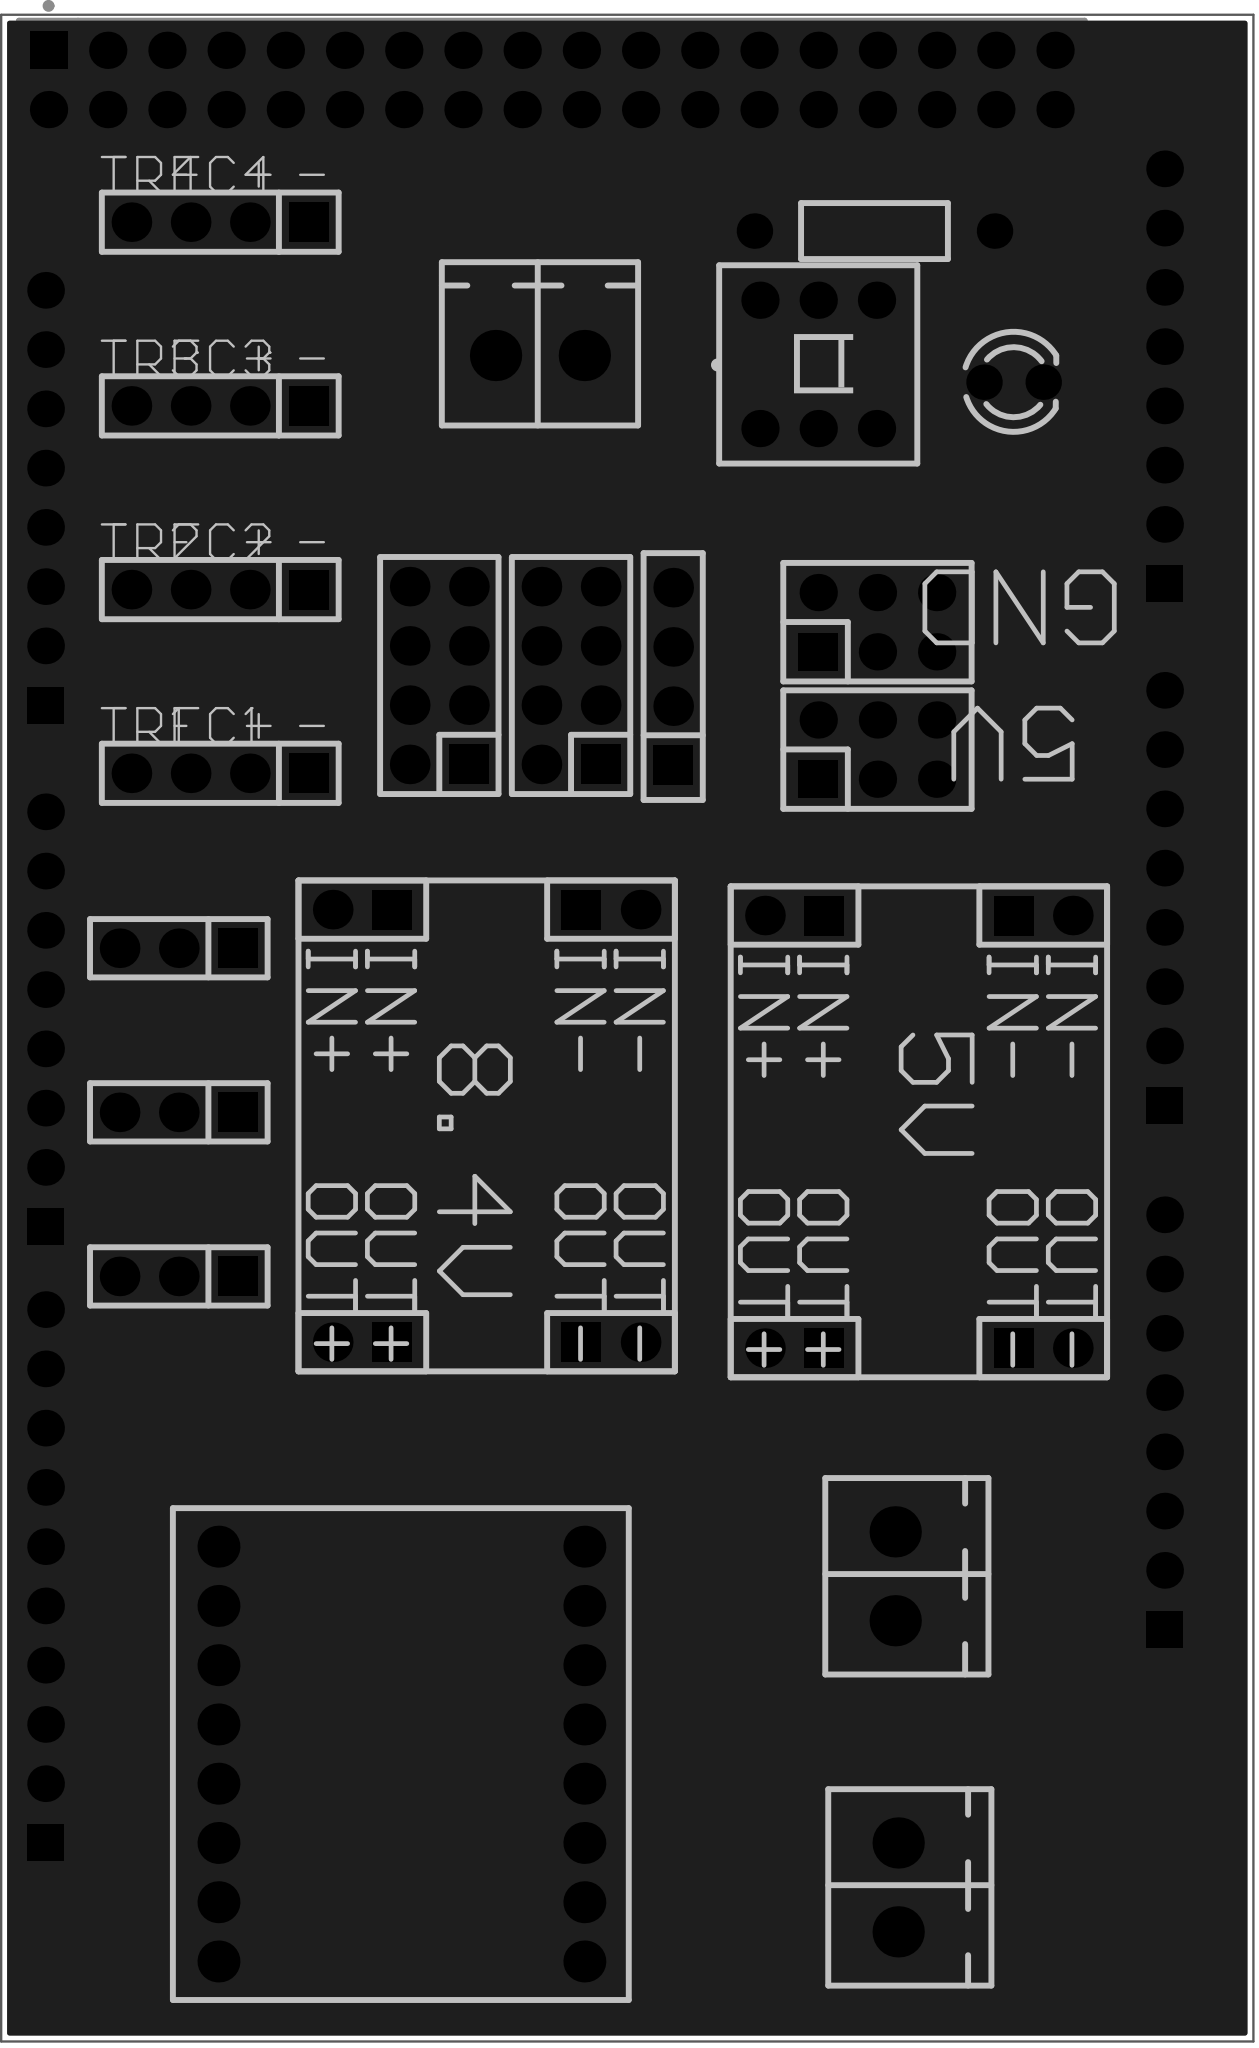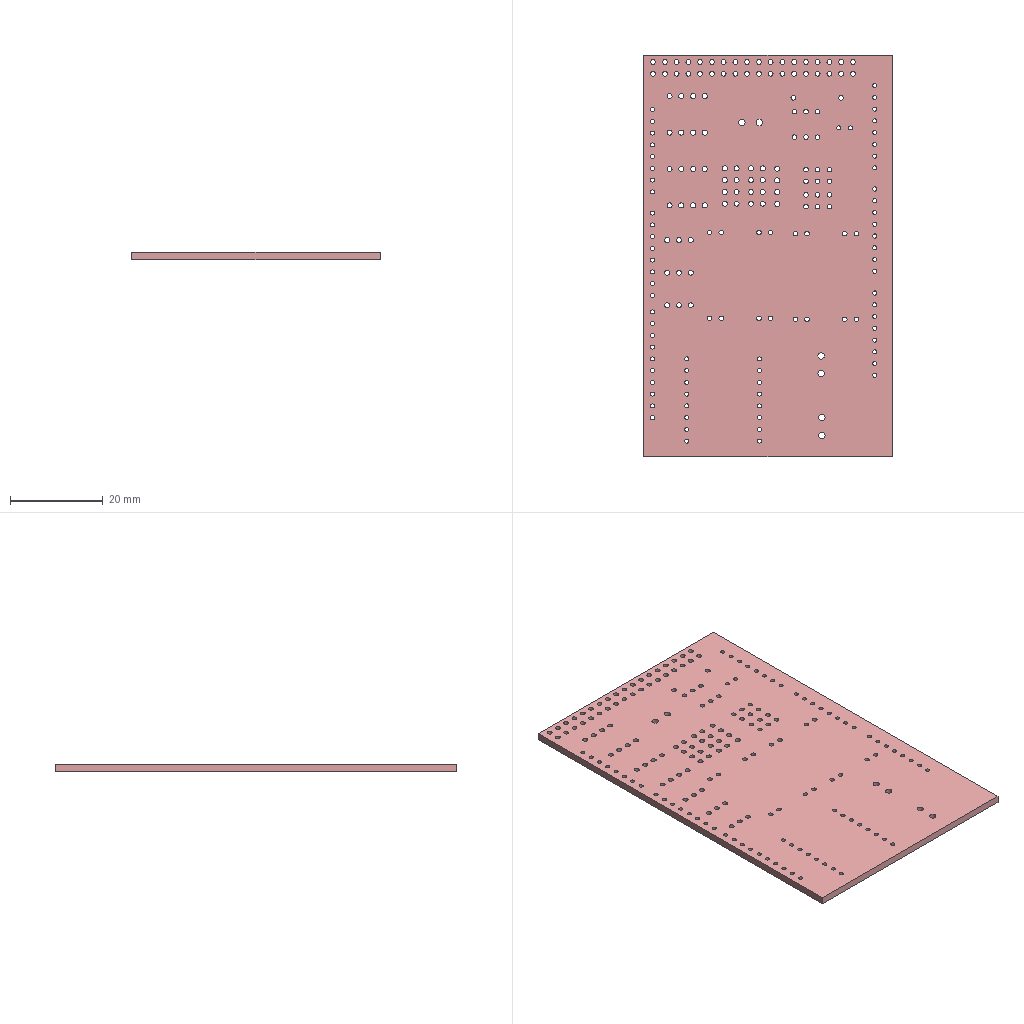Circuit board layout | Altium Designer | box 53.7 x 86.9 x 1.6 mm
Layer stack:
# Altium Designer layer stack of  (unit mm; dielectric type: 0 none, 1 core, 2 prepreg, 3 surface material)
index,name,kind,layer,copper_thickness_mm,dielectric_type,dielectric_thickness_mm,dielectric_material,dielectric_constant
0,Top Paste Mask Layer,other,,,,,,
1,Top Silkscreen Layer,other,,,,,,
2,Top Solder Mask Layer,dielectric,,,3,0.01,,3.3
3,Top Layer,copper,Top Layer,0.035,,,,
4,Dielectric1,dielectric,,,3,1.51,FR4,4.5
5,Bottom Layer,copper,Bottom Layer,0.035,,,,
6,Bottom Solder Mask Layer,dielectric,,,3,0.01,,3.3
7,Bottom Silkscreen Layer,other,,,,,,
8,Bottom Paste Mask Layer,other,,,,,,
# drill layer pairs: low layer,high layer
drill_pair,Top Layer,Bottom Layer
Part placement:
Designator,Comment,Layer,Footprint,Center-X(mm),Center-Y(mm),Rotation
H3,,TopLayer,HDR-TH_8P-P2.54-V-M,104.14,123.698,270
H6,,TopLayer,HDR-TH_8P-P2.54-V-M-R2-C4-S2.54,102.108,143.002,90
H7,,TopLayer,HDR-TH_8P-P2.54-V-M-R2-C4-S2.54,107.76,143.002,90
H8,,TopLayer,HDR-TH_4P-P2.54-V-F,112.141,142.958,90
H9,,TopLayer,HDR-TH_3P-P2.54-V-M,90.932,117.247,180
H10,,TopLayer,HDR-TH_3P-P2.54-V-M,90.932,124.28,180
H11,,TopLayer,HDR-TH_3P-P2.54-V-M,90.932,131.313,180
H12,,TopLayer,HDR-TH_8P-P2.54-V-M,122.682,123.444,270
H13,,TopLayer,HDR-TH_6P-P2.54-V-F-R2-C3-S2.54,120.904,139.827,0
H14,,TopLayer,HDR-TH_6P-P2.54-V-F-R2-C3-S2.54,120.904,145.288,0
H15,,TopLayer,HDR-TH_4P-P2.54-V-M,92.71,138.811,180
H16,,TopLayer,HDR-TH_4P-P2.54-V-M,92.71,146.685,180
H17,,TopLayer,HDR-TH_4P-P2.54-V-M,92.71,154.559,180
H18,,TopLayer,HDR-TH_4P-P2.54-V-M,92.71,162.433,180
KEY1,Self-locking switch,TopLayer,SW-TH_6P-L8.5-W8.5-P2.54,118.364,156.337,0
LED1,,TopLayer,LED_TH-3mm,126.746,155.575,0
R1,1kΩ,TopLayer,Res_1/4W,120.777,162.052,180
U1,2P-P3.81_KF2EDGV-3.81-2P,TopLayer,CONN-TH_2P-P3.81_KF2EDGV-3.81-2P,106.426,156.718,180
U3,,BottomLayer,tb6612,100.482,96.774,180
U4,2P-P3.81_KF2EDGV-3.81-2P,TopLayer,CONN-TH_2P-P3.81_KF2EDGV-3.81-2P,121.666,104.394,90
U5,2P-P3.81_KF2EDGV-3.81-2P,TopLayer,CONN-TH_2P-P3.81_KF2EDGV-3.81-2P,121.793,91.059,90
H19,X6521WV-2×18H-C30D60,BottomLayer,HDR-TH_36P-2.54-V-M-R2-C18-S2.54,106.934,168.529,0
J1,3-way TX/RX,BottomLayer,HDR-M-2.54_1X8,85.217,150.622,90
J2,PWM D2~D7,BottomLayer,HDR-M-2.54_1X8,85.217,128.27,90
J4,PWM_D8~D13,BottomLayer,HDR-M-2.54_1X10,85.217,104.394,90
J8,HDR-M-2.54_1x8,BottomLayer,HDR-M-2.54_1X8,133.223,133.477,90
J9,HDR-M-2.54_1x8,BottomLayer,HDR-M-2.54_1X8,133.223,110.998,90
J14,HDR-M-2.54_1x8,BottomLayer,HDR-M-2.54_1X8,133.223,155.829,90
Pad and via stacks:
# Altium Designer via and pad stacks of  (unit mm). Each distinct definition once, with the count of objects using it.
# via: kind,start_layer,end_layer,hole_mm,diameter_mm,mode(0 simple;1 top-mid-bottom;2 full stack),diameter_per_layer,count,example_net
# pad: kind,layer,hole_mm,hole_type(0 round;1 square;2 slot),plating,top_size,top_shape(1 round;2 rect;3 octagon;9 rounded rect),mid_size,bottom_size,mode,footprint,size_per_layer,count,example
pad,Multi-Layer,1,0,plated,1.7x1.7,2,1.7x1.7,1.7x1.7,0,HDR-TH_8P-P2.54-V-M,,8,H3.2
pad,Multi-Layer,1,0,plated,1.7x1.7,1,1.7x1.7,1.7x1.7,0,HDR-TH_8P-P2.54-V-M,,8,H3.1
pad,Multi-Layer,1.1,0,plated,1.7x1.7,2,1.7x1.7,1.7x1.7,0,HDR-TH_8P-P2.54-V-M-R2-C4-S2.54,,2,H6.1
pad,Multi-Layer,1.1,0,plated,1.7x1.7,1,1.7x1.7,1.7x1.7,0,HDR-TH_8P-P2.54-V-M-R2-C4-S2.54,,14,H6.2
pad,Multi-Layer,1.1,0,plated,1.7x1.7,2,1.7x1.7,1.7x1.7,0,HDR-TH_4P-P2.54-V-F,,1,H8.1
pad,Multi-Layer,1.1,0,plated,1.7x1.7,1,1.7x1.7,1.7x1.7,0,HDR-TH_4P-P2.54-V-F,,3,H8.2
pad,Multi-Layer,1.1,0,plated,1.7x1.7,2,1.7x1.7,1.7x1.7,0,HDR-TH_3P-P2.54-V-M,,3,H9.1
pad,Multi-Layer,1.1,0,plated,1.7x1.7,1,1.7x1.7,1.7x1.7,0,HDR-TH_3P-P2.54-V-M,,6,H9.2
pad,Multi-Layer,1,0,plated,1.7x1.6,2,1.7x1.6,1.7x1.6,0,HDR-TH_6P-P2.54-V-F-R2-C3-S2.54,,2,H13.1
pad,Multi-Layer,1,0,plated,1.6x1.6,1,1.6x1.6,1.6x1.6,0,HDR-TH_6P-P2.54-V-F-R2-C3-S2.54,,10,H13.2
pad,Multi-Layer,1.1,0,plated,1.7x1.7,2,1.7x1.7,1.7x1.7,0,HDR-TH_4P-P2.54-V-M,,4,H15.1
pad,Multi-Layer,1.1,0,plated,1.7x1.7,1,1.7x1.7,1.7x1.7,0,HDR-TH_4P-P2.54-V-M,,12,H15.2
pad,Multi-Layer,1,0,plated,1.6x1.6,1,1.6x1.6,1.6x1.6,0,SW-TH_6P-L8.5-W8.5-P2.54,,6,KEY1.4
pad,Multi-Layer,0.9144,0,plated,1.524x1.524,1,1.524x1.524,1.524x1.524,0,LED_TH-3mm,,2,LED1.1
pad,Multi-Layer,1,0,plated,1.524x1.524,1,1.524x1.524,1.524x1.524,0,Res_1/4W,,2,R1.1
pad,Multi-Layer,1.4,0,plated,2.2x2.2,1,2.2x2.2,2.2x2.2,0,CONN-TH_2P-P3.81_KF2EDGV-3.81-2P,,6,U1.2
pad,Multi-Layer,0.9,0,plated,1.8x1.8,1,1.8x1.8,1.8x1.8,0,tb6612,,16,U3.1
pad,Multi-Layer,1.05,0,plated,1.6x1.6,2,1.6x1.6,1.6x1.6,0,HDR-TH_36P-2.54-V-M-R2-C18-S2.54,,1,H19.1
pad,Multi-Layer,1.05,0,plated,1.6x1.6,1,1.6x1.6,1.6x1.6,0,HDR-TH_36P-2.54-V-M-R2-C18-S2.54,,35,H19.2
pad,Multi-Layer,0.889,0,plated,1.575x1.575,2,1.575x1.575,1.575x1.575,0,HDR-M-2.54_1X8,,5,J1.1
pad,Multi-Layer,0.889,0,plated,1.575x1.575,1,1.575x1.575,1.575x1.575,0,HDR-M-2.54_1X8,,35,J1.2
pad,Multi-Layer,0.889,0,plated,1.575x1.575,1,1.575x1.575,1.575x1.575,0,HDR-M-2.54_1X10,,9,J4.10
pad,Multi-Layer,0.9449,0,plated,1.575x1.575,2,1.575x1.575,1.575x1.575,0,HDR-M-2.54_1X10,,1,J4.1
Copper pours:
name,layer,net,type(0 solid;1 hatched;2 none)
Top Layer-GND,Top Layer,GND,0
Bottom Layer-GND,Bottom Layer,GND,0